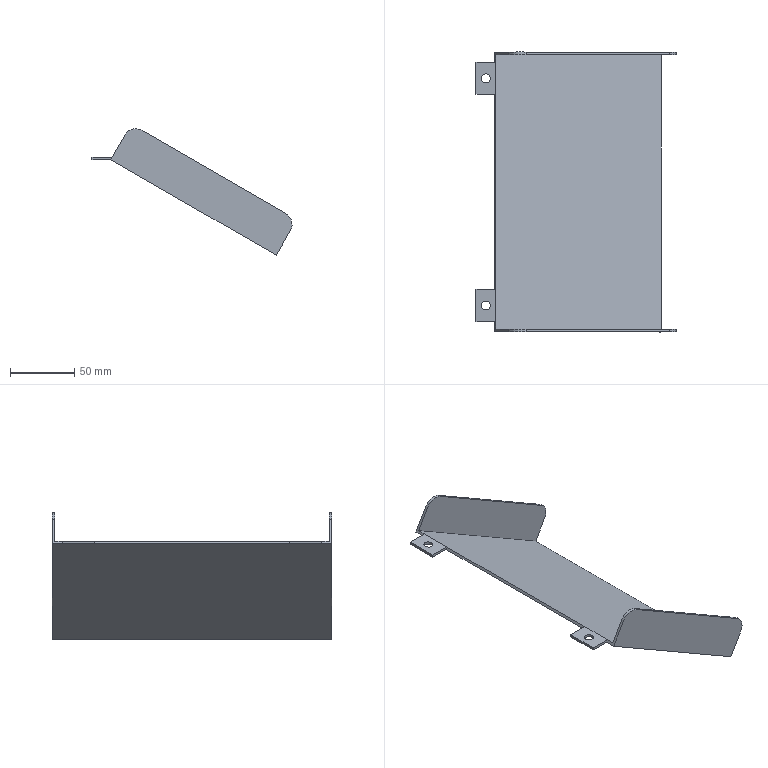Part | NX | features solid 2 | 1 solid | 30 faces | box 155.867 x 218 x 98.525 mm | volume 83984 mm3 | plane 24 | cylinder 6 | commonest cylinder face diameters 20 x4 7 x2
STEP:
#1=CARTESIAN_POINT('',(829.555,109.,-46.232));
#2=VERTEX_POINT('',#1);
#3=CARTESIAN_POINT('',(829.555,101.,-46.232));
#4=VERTEX_POINT('',#3);
#5=CARTESIAN_POINT('',(829.555,135.,-46.232));
#6=DIRECTION('',(0.,-1.,0.));
#7=VECTOR('',#6,1000.);
#8=LINE('',#5,#7);
#9=EDGE_CURVE('',#2,#4,#8,.T.);
#10=ORIENTED_EDGE('',*,*,#9,.T.);
#11=CARTESIAN_POINT('',(830.555,101.,-44.5));
#12=VERTEX_POINT('',#11);
#13=CARTESIAN_POINT('',(829.555,101.,-46.232));
#14=DIRECTION('',(-0.5,0.,-0.866));
#15=VECTOR('',#14,1000.);
#16=LINE('',#13,#15);
#17=EDGE_CURVE('',#4,#12,#16,.F.);
#18=ORIENTED_EDGE('',*,*,#17,.T.);
#19=CARTESIAN_POINT('',(830.555,107.,-44.5));
#20=VERTEX_POINT('',#19);
#21=CARTESIAN_POINT('',(830.555,135.,-44.5));
#22=DIRECTION('',(0.,-1.,0.));
#23=VECTOR('',#22,1000.);
#24=LINE('',#21,#23);
#25=EDGE_CURVE('',#20,#12,#24,.T.);
#26=ORIENTED_EDGE('',*,*,#25,.F.);
#27=CARTESIAN_POINT('',(840.555,107.,-27.179));
#28=VERTEX_POINT('',#27);
#29=CARTESIAN_POINT('',(830.555,107.,-44.5));
#30=DIRECTION('',(-0.5,0.,-0.866));
#31=VECTOR('',#30,1000.);
#32=LINE('',#29,#31);
#33=EDGE_CURVE('',#28,#20,#32,.T.);
#34=ORIENTED_EDGE('',*,*,#33,.F.);
#35=CARTESIAN_POINT('',(840.555,109.,-27.179));
#36=VERTEX_POINT('',#35);
#37=CARTESIAN_POINT('',(840.555,109.,-27.179));
#38=DIRECTION('',(0.,1.,0.));
#39=VECTOR('',#38,1000.);
#40=LINE('',#37,#39);
#41=EDGE_CURVE('',#28,#36,#40,.T.);
#42=ORIENTED_EDGE('',*,*,#41,.T.);
#43=CARTESIAN_POINT('',(830.555,109.,-44.5));
#44=DIRECTION('',(-0.5,0.,-0.866));
#45=VECTOR('',#44,1000.);
#46=LINE('',#43,#45);
#47=EDGE_CURVE('',#36,#2,#46,.T.);
#48=ORIENTED_EDGE('',*,*,#47,.T.);
#49=EDGE_LOOP('',(#10,#18,#26,#34,#42,#48));
#50=FACE_BOUND('',#49,.T.);
#51=CARTESIAN_POINT('',(829.555,99.,-46.232));
#52=DIRECTION('',(-0.866,0.,0.5));
#53=DIRECTION('',(0.5,0.,0.866));
#54=AXIS2_PLACEMENT_3D('',#51,#52,#53);
#55=PLANE('',#54);
#56=ADVANCED_FACE('',(#50),#55,.T.);
#57=CARTESIAN_POINT('',(829.555,76.,-46.232));
#58=VERTEX_POINT('',#57);
#59=CARTESIAN_POINT('',(830.555,76.,-44.5));
#60=VERTEX_POINT('',#59);
#61=CARTESIAN_POINT('',(827.39,76.,-49.982));
#62=DIRECTION('',(-0.5,0.,-0.866));
#63=VECTOR('',#62,1000.);
#64=LINE('',#61,#63);
#65=EDGE_CURVE('',#58,#60,#64,.F.);
#66=ORIENTED_EDGE('',*,*,#65,.F.);
#67=CARTESIAN_POINT('',(829.555,-76.,-46.232));
#68=VERTEX_POINT('',#67);
#69=CARTESIAN_POINT('',(829.555,135.,-46.232));
#70=DIRECTION('',(0.,-1.,0.));
#71=VECTOR('',#70,1000.);
#72=LINE('',#69,#71);
#73=EDGE_CURVE('',#58,#68,#72,.T.);
#74=ORIENTED_EDGE('',*,*,#73,.T.);
#75=CARTESIAN_POINT('',(830.555,-76.,-44.5));
#76=VERTEX_POINT('',#75);
#77=CARTESIAN_POINT('',(827.39,-76.,-49.982));
#78=DIRECTION('',(-0.5,0.,-0.866));
#79=VECTOR('',#78,1000.);
#80=LINE('',#77,#79);
#81=EDGE_CURVE('',#68,#76,#80,.F.);
#82=ORIENTED_EDGE('',*,*,#81,.T.);
#83=CARTESIAN_POINT('',(830.555,135.,-44.5));
#84=DIRECTION('',(0.,-1.,0.));
#85=VECTOR('',#84,1000.);
#86=LINE('',#83,#85);
#87=EDGE_CURVE('',#60,#76,#86,.T.);
#88=ORIENTED_EDGE('',*,*,#87,.F.);
#89=EDGE_LOOP('',(#66,#74,#82,#88));
#90=FACE_BOUND('',#89,.T.);
#91=CARTESIAN_POINT('',(829.555,99.,-46.232));
#92=DIRECTION('',(-0.866,0.,0.5));
#93=DIRECTION('',(0.5,0.,0.866));
#94=AXIS2_PLACEMENT_3D('',#91,#92,#93);
#95=PLANE('',#94);
#96=ADVANCED_FACE('',(#90),#95,.T.);
#97=ORIENTED_EDGE('',*,*,#47,.F.);
#98=CARTESIAN_POINT('',(854.215,109.,-23.519));
#99=VERTEX_POINT('',#98);
#100=CARTESIAN_POINT('',(849.215,109.,-32.179));
#101=DIRECTION('',(0.,-1.,0.));
#102=DIRECTION('',(0.,0.,-1.));
#103=AXIS2_PLACEMENT_3D('',#100,#101,#102);
#104=CIRCLE('',#103,10.);
#105=EDGE_CURVE('',#36,#99,#104,.F.);
#106=ORIENTED_EDGE('',*,*,#105,.T.);
#107=CARTESIAN_POINT('',(965.886,109.,-87.992));
#108=VERTEX_POINT('',#107);
#109=CARTESIAN_POINT('',(713.006,109.,58.008));
#110=DIRECTION('',(0.866,0.,-0.5));
#111=VECTOR('',#110,1000.);
#112=LINE('',#109,#111);
#113=EDGE_CURVE('',#99,#108,#112,.T.);
#114=ORIENTED_EDGE('',*,*,#113,.T.);
#115=CARTESIAN_POINT('',(969.546,109.,-101.652));
#116=VERTEX_POINT('',#115);
#117=CARTESIAN_POINT('',(960.886,109.,-96.652));
#118=DIRECTION('',(0.,-1.,0.));
#119=DIRECTION('',(0.08716,0.,0.9962));
#120=AXIS2_PLACEMENT_3D('',#117,#118,#119);
#121=CIRCLE('',#120,10.);
#122=EDGE_CURVE('',#108,#116,#121,.F.);
#123=ORIENTED_EDGE('',*,*,#122,.T.);
#124=CARTESIAN_POINT('',(958.546,109.,-120.705));
#125=VERTEX_POINT('',#124);
#126=CARTESIAN_POINT('',(959.546,109.,-118.973));
#127=DIRECTION('',(-0.5,0.,-0.866));
#128=VECTOR('',#127,1000.);
#129=LINE('',#126,#128);
#130=EDGE_CURVE('',#116,#125,#129,.T.);
#131=ORIENTED_EDGE('',*,*,#130,.T.);
#132=CARTESIAN_POINT('',(697.006,109.,30.295));
#133=DIRECTION('',(-0.866,0.,0.5));
#134=VECTOR('',#133,1000.);
#135=LINE('',#132,#134);
#136=EDGE_CURVE('',#125,#2,#135,.T.);
#137=ORIENTED_EDGE('',*,*,#136,.T.);
#138=EDGE_LOOP('',(#97,#106,#114,#123,#131,#137));
#139=FACE_BOUND('',#138,.T.);
#140=CARTESIAN_POINT('',(698.006,109.,32.027));
#141=DIRECTION('',(0.,-1.,0.));
#142=DIRECTION('',(0.08716,0.,0.9962));
#143=AXIS2_PLACEMENT_3D('',#140,#141,#142);
#144=PLANE('',#143);
#145=ADVANCED_FACE('',(#139),#144,.F.);
#146=CARTESIAN_POINT('',(854.215,-109.,-23.519));
#147=VERTEX_POINT('',#146);
#148=CARTESIAN_POINT('',(965.886,-109.,-87.992));
#149=VERTEX_POINT('',#148);
#150=CARTESIAN_POINT('',(713.006,-109.,58.008));
#151=DIRECTION('',(0.866,0.,-0.5));
#152=VECTOR('',#151,1000.);
#153=LINE('',#150,#152);
#154=EDGE_CURVE('',#147,#149,#153,.T.);
#155=ORIENTED_EDGE('',*,*,#154,.F.);
#156=CARTESIAN_POINT('',(840.555,-109.,-27.179));
#157=VERTEX_POINT('',#156);
#158=CARTESIAN_POINT('',(849.215,-109.,-32.179));
#159=DIRECTION('',(0.,1.,0.));
#160=DIRECTION('',(0.,0.,1.));
#161=AXIS2_PLACEMENT_3D('',#158,#159,#160);
#162=CIRCLE('',#161,10.);
#163=EDGE_CURVE('',#147,#157,#162,.F.);
#164=ORIENTED_EDGE('',*,*,#163,.T.);
#165=CARTESIAN_POINT('',(829.555,-109.,-46.232));
#166=VERTEX_POINT('',#165);
#167=CARTESIAN_POINT('',(830.555,-109.,-44.5));
#168=DIRECTION('',(0.5,0.,0.866));
#169=VECTOR('',#168,1000.);
#170=LINE('',#167,#169);
#171=EDGE_CURVE('',#166,#157,#170,.T.);
#172=ORIENTED_EDGE('',*,*,#171,.F.);
#173=CARTESIAN_POINT('',(958.546,-109.,-120.705));
#174=VERTEX_POINT('',#173);
#175=CARTESIAN_POINT('',(697.006,-109.,30.295));
#176=DIRECTION('',(0.866,0.,-0.5));
#177=VECTOR('',#176,1000.);
#178=LINE('',#175,#177);
#179=EDGE_CURVE('',#166,#174,#178,.T.);
#180=ORIENTED_EDGE('',*,*,#179,.T.);
#181=CARTESIAN_POINT('',(969.546,-109.,-101.652));
#182=VERTEX_POINT('',#181);
#183=CARTESIAN_POINT('',(959.546,-109.,-118.973));
#184=DIRECTION('',(-0.5,0.,-0.866));
#185=VECTOR('',#184,1000.);
#186=LINE('',#183,#185);
#187=EDGE_CURVE('',#182,#174,#186,.T.);
#188=ORIENTED_EDGE('',*,*,#187,.F.);
#189=CARTESIAN_POINT('',(960.886,-109.,-96.652));
#190=DIRECTION('',(0.,1.,0.));
#191=DIRECTION('',(-0.08716,0.,-0.9962));
#192=AXIS2_PLACEMENT_3D('',#189,#190,#191);
#193=CIRCLE('',#192,10.);
#194=EDGE_CURVE('',#182,#149,#193,.F.);
#195=ORIENTED_EDGE('',*,*,#194,.T.);
#196=EDGE_LOOP('',(#155,#164,#172,#180,#188,#195));
#197=FACE_BOUND('',#196,.T.);
#198=CARTESIAN_POINT('',(698.006,-109.,32.027));
#199=DIRECTION('',(0.,1.,0.));
#200=DIRECTION('',(-0.08716,0.,-0.9962));
#201=AXIS2_PLACEMENT_3D('',#198,#199,#200);
#202=PLANE('',#201);
#203=ADVANCED_FACE('',(#197),#202,.F.);
#204=CARTESIAN_POINT('',(830.555,-107.,-44.5));
#205=VERTEX_POINT('',#204);
#206=CARTESIAN_POINT('',(840.555,-107.,-27.179));
#207=VERTEX_POINT('',#206);
#208=CARTESIAN_POINT('',(830.555,-107.,-44.5));
#209=DIRECTION('',(0.5,0.,0.866));
#210=VECTOR('',#209,1000.);
#211=LINE('',#208,#210);
#212=EDGE_CURVE('',#205,#207,#211,.T.);
#213=ORIENTED_EDGE('',*,*,#212,.T.);
#214=CARTESIAN_POINT('',(854.215,-107.,-23.519));
#215=VERTEX_POINT('',#214);
#216=CARTESIAN_POINT('',(849.215,-107.,-32.179));
#217=DIRECTION('',(0.,1.,0.));
#218=DIRECTION('',(0.,0.,1.));
#219=AXIS2_PLACEMENT_3D('',#216,#217,#218);
#220=CIRCLE('',#219,10.);
#221=EDGE_CURVE('',#207,#215,#220,.T.);
#222=ORIENTED_EDGE('',*,*,#221,.T.);
#223=CARTESIAN_POINT('',(965.886,-107.,-87.992));
#224=VERTEX_POINT('',#223);
#225=CARTESIAN_POINT('',(713.006,-107.,58.008));
#226=DIRECTION('',(0.866,0.,-0.5));
#227=VECTOR('',#226,1000.);
#228=LINE('',#225,#227);
#229=EDGE_CURVE('',#215,#224,#228,.T.);
#230=ORIENTED_EDGE('',*,*,#229,.T.);
#231=CARTESIAN_POINT('',(969.546,-107.,-101.652));
#232=VERTEX_POINT('',#231);
#233=CARTESIAN_POINT('',(960.886,-107.,-96.652));
#234=DIRECTION('',(0.,1.,0.));
#235=DIRECTION('',(-0.08716,0.,-0.9962));
#236=AXIS2_PLACEMENT_3D('',#233,#234,#235);
#237=CIRCLE('',#236,10.);
#238=EDGE_CURVE('',#224,#232,#237,.T.);
#239=ORIENTED_EDGE('',*,*,#238,.T.);
#240=CARTESIAN_POINT('',(959.546,-107.,-118.973));
#241=VERTEX_POINT('',#240);
#242=CARTESIAN_POINT('',(959.546,-107.,-118.973));
#243=DIRECTION('',(-0.5,0.,-0.866));
#244=VECTOR('',#243,1000.);
#245=LINE('',#242,#244);
#246=EDGE_CURVE('',#232,#241,#245,.T.);
#247=ORIENTED_EDGE('',*,*,#246,.T.);
#248=CARTESIAN_POINT('',(698.006,-107.,32.027));
#249=DIRECTION('',(-0.866,0.,0.5));
#250=VECTOR('',#249,1000.);
#251=LINE('',#248,#250);
#252=EDGE_CURVE('',#241,#205,#251,.T.);
#253=ORIENTED_EDGE('',*,*,#252,.T.);
#254=EDGE_LOOP('',(#213,#222,#230,#239,#247,#253));
#255=FACE_BOUND('',#254,.T.);
#256=CARTESIAN_POINT('',(698.006,-107.,32.027));
#257=DIRECTION('',(0.,1.,0.));
#258=DIRECTION('',(-0.08716,0.,-0.9962));
#259=AXIS2_PLACEMENT_3D('',#256,#257,#258);
#260=PLANE('',#259);
#261=ADVANCED_FACE('',(#255),#260,.T.);
#262=CARTESIAN_POINT('',(854.215,107.,-23.519));
#263=VERTEX_POINT('',#262);
#264=CARTESIAN_POINT('',(965.886,107.,-87.992));
#265=VERTEX_POINT('',#264);
#266=CARTESIAN_POINT('',(713.006,107.,58.008));
#267=DIRECTION('',(0.866,0.,-0.5));
#268=VECTOR('',#267,1000.);
#269=LINE('',#266,#268);
#270=EDGE_CURVE('',#263,#265,#269,.T.);
#271=ORIENTED_EDGE('',*,*,#270,.F.);
#272=CARTESIAN_POINT('',(849.215,107.,-32.179));
#273=DIRECTION('',(0.,-1.,0.));
#274=DIRECTION('',(0.,0.,-1.));
#275=AXIS2_PLACEMENT_3D('',#272,#273,#274);
#276=CIRCLE('',#275,10.);
#277=EDGE_CURVE('',#263,#28,#276,.T.);
#278=ORIENTED_EDGE('',*,*,#277,.T.);
#279=ORIENTED_EDGE('',*,*,#33,.T.);
#280=CARTESIAN_POINT('',(959.546,107.,-118.973));
#281=VERTEX_POINT('',#280);
#282=CARTESIAN_POINT('',(698.006,107.,32.027));
#283=DIRECTION('',(0.866,0.,-0.5));
#284=VECTOR('',#283,1000.);
#285=LINE('',#282,#284);
#286=EDGE_CURVE('',#20,#281,#285,.T.);
#287=ORIENTED_EDGE('',*,*,#286,.T.);
#288=CARTESIAN_POINT('',(969.546,107.,-101.652));
#289=VERTEX_POINT('',#288);
#290=CARTESIAN_POINT('',(959.546,107.,-118.973));
#291=DIRECTION('',(-0.5,0.,-0.866));
#292=VECTOR('',#291,1000.);
#293=LINE('',#290,#292);
#294=EDGE_CURVE('',#289,#281,#293,.T.);
#295=ORIENTED_EDGE('',*,*,#294,.F.);
#296=CARTESIAN_POINT('',(960.886,107.,-96.652));
#297=DIRECTION('',(0.,-1.,0.));
#298=DIRECTION('',(0.08716,0.,0.9962));
#299=AXIS2_PLACEMENT_3D('',#296,#297,#298);
#300=CIRCLE('',#299,10.);
#301=EDGE_CURVE('',#289,#265,#300,.T.);
#302=ORIENTED_EDGE('',*,*,#301,.T.);
#303=EDGE_LOOP('',(#271,#278,#279,#287,#295,#302));
#304=FACE_BOUND('',#303,.T.);
#305=CARTESIAN_POINT('',(698.006,107.,32.027));
#306=DIRECTION('',(0.,-1.,0.));
#307=DIRECTION('',(-0.08716,0.,-0.9962));
#308=AXIS2_PLACEMENT_3D('',#305,#306,#307);
#309=PLANE('',#308);
#310=ADVANCED_FACE('',(#304),#309,.T.);
#311=ORIENTED_EDGE('',*,*,#229,.F.);
#312=CARTESIAN_POINT('',(854.215,-109.,-23.519));
#313=DIRECTION('',(0.,1.,0.));
#314=VECTOR('',#313,1000.);
#315=LINE('',#312,#314);
#316=EDGE_CURVE('',#215,#147,#315,.F.);
#317=ORIENTED_EDGE('',*,*,#316,.T.);
#318=ORIENTED_EDGE('',*,*,#154,.T.);
#319=CARTESIAN_POINT('',(965.886,-107.,-87.992));
#320=DIRECTION('',(0.,-1.,0.));
#321=VECTOR('',#320,1000.);
#322=LINE('',#319,#321);
#323=EDGE_CURVE('',#149,#224,#322,.F.);
#324=ORIENTED_EDGE('',*,*,#323,.T.);
#325=EDGE_LOOP('',(#311,#317,#318,#324));
#326=FACE_BOUND('',#325,.T.);
#327=CARTESIAN_POINT('',(713.006,-107.,58.008));
#328=DIRECTION('',(-0.5,0.,-0.866));
#329=DIRECTION('',(-0.866,0.,0.5));
#330=AXIS2_PLACEMENT_3D('',#327,#328,#329);
#331=PLANE('',#330);
#332=ADVANCED_FACE('',(#326),#331,.F.);
#333=ORIENTED_EDGE('',*,*,#113,.F.);
#334=CARTESIAN_POINT('',(854.215,107.,-23.519));
#335=DIRECTION('',(0.,1.,0.));
#336=VECTOR('',#335,1000.);
#337=LINE('',#334,#336);
#338=EDGE_CURVE('',#99,#263,#337,.F.);
#339=ORIENTED_EDGE('',*,*,#338,.T.);
#340=ORIENTED_EDGE('',*,*,#270,.T.);
#341=CARTESIAN_POINT('',(965.886,107.,-87.992));
#342=DIRECTION('',(0.,1.,0.));
#343=VECTOR('',#342,1000.);
#344=LINE('',#341,#343);
#345=EDGE_CURVE('',#265,#108,#344,.T.);
#346=ORIENTED_EDGE('',*,*,#345,.T.);
#347=EDGE_LOOP('',(#333,#339,#340,#346));
#348=FACE_BOUND('',#347,.T.);
#349=CARTESIAN_POINT('',(713.006,107.,58.008));
#350=DIRECTION('',(-0.5,0.,-0.866));
#351=DIRECTION('',(-0.866,0.,0.5));
#352=AXIS2_PLACEMENT_3D('',#349,#350,#351);
#353=PLANE('',#352);
#354=ADVANCED_FACE('',(#348),#353,.F.);
#355=ORIENTED_EDGE('',*,*,#286,.F.);
#356=ORIENTED_EDGE('',*,*,#25,.T.);
#357=CARTESIAN_POINT('',(830.555,99.,-44.5));
#358=DIRECTION('',(0.,1.,0.));
#359=VECTOR('',#358,1000.);
#360=LINE('',#357,#359);
#361=EDGE_CURVE('',#12,#60,#360,.F.);
#362=ORIENTED_EDGE('',*,*,#361,.T.);
#363=ORIENTED_EDGE('',*,*,#87,.T.);
#364=CARTESIAN_POINT('',(830.555,-101.,-44.5));
#365=VERTEX_POINT('',#364);
#366=CARTESIAN_POINT('',(830.555,-99.,-44.5));
#367=DIRECTION('',(0.,-1.,0.));
#368=VECTOR('',#367,1000.);
#369=LINE('',#366,#368);
#370=EDGE_CURVE('',#365,#76,#369,.F.);
#371=ORIENTED_EDGE('',*,*,#370,.F.);
#372=CARTESIAN_POINT('',(830.555,135.,-44.5));
#373=DIRECTION('',(0.,-1.,0.));
#374=VECTOR('',#373,1000.);
#375=LINE('',#372,#374);
#376=EDGE_CURVE('',#365,#205,#375,.T.);
#377=ORIENTED_EDGE('',*,*,#376,.T.);
#378=ORIENTED_EDGE('',*,*,#252,.F.);
#379=CARTESIAN_POINT('',(959.546,135.,-118.973));
#380=DIRECTION('',(0.,-1.,0.));
#381=VECTOR('',#380,1000.);
#382=LINE('',#379,#381);
#383=EDGE_CURVE('',#241,#281,#382,.F.);
#384=ORIENTED_EDGE('',*,*,#383,.T.);
#385=EDGE_LOOP('',(#355,#356,#362,#363,#371,#377,#378,#384));
#386=FACE_BOUND('',#385,.T.);
#387=CARTESIAN_POINT('',(698.006,135.,32.027));
#388=DIRECTION('',(0.5,0.,0.866));
#389=DIRECTION('',(0.,1.,0.));
#390=AXIS2_PLACEMENT_3D('',#387,#388,#389);
#391=PLANE('',#390);
#392=ADVANCED_FACE('',(#386),#391,.T.);
#393=ORIENTED_EDGE('',*,*,#9,.F.);
#394=ORIENTED_EDGE('',*,*,#136,.F.);
#395=CARTESIAN_POINT('',(958.546,135.,-120.705));
#396=DIRECTION('',(0.,-1.,0.));
#397=VECTOR('',#396,1000.);
#398=LINE('',#395,#397);
#399=EDGE_CURVE('',#174,#125,#398,.F.);
#400=ORIENTED_EDGE('',*,*,#399,.F.);
#401=ORIENTED_EDGE('',*,*,#179,.F.);
#402=CARTESIAN_POINT('',(829.555,-101.,-46.232));
#403=VERTEX_POINT('',#402);
#404=CARTESIAN_POINT('',(829.555,135.,-46.232));
#405=DIRECTION('',(0.,-1.,0.));
#406=VECTOR('',#405,1000.);
#407=LINE('',#404,#406);
#408=EDGE_CURVE('',#403,#166,#407,.T.);
#409=ORIENTED_EDGE('',*,*,#408,.F.);
#410=CARTESIAN_POINT('',(829.555,135.,-46.232));
#411=DIRECTION('',(0.,-1.,0.));
#412=VECTOR('',#411,1000.);
#413=LINE('',#410,#412);
#414=EDGE_CURVE('',#68,#403,#413,.T.);
#415=ORIENTED_EDGE('',*,*,#414,.F.);
#416=ORIENTED_EDGE('',*,*,#73,.F.);
#417=CARTESIAN_POINT('',(829.555,135.,-46.232));
#418=DIRECTION('',(0.,-1.,0.));
#419=VECTOR('',#418,1000.);
#420=LINE('',#417,#419);
#421=EDGE_CURVE('',#4,#58,#420,.T.);
#422=ORIENTED_EDGE('',*,*,#421,.F.);
#423=EDGE_LOOP('',(#393,#394,#400,#401,#409,#415,#416,#422));
#424=FACE_BOUND('',#423,.T.);
#425=CARTESIAN_POINT('',(697.006,135.,30.295));
#426=DIRECTION('',(0.5,0.,0.866));
#427=DIRECTION('',(0.,1.,0.));
#428=AXIS2_PLACEMENT_3D('',#425,#426,#427);
#429=PLANE('',#428);
#430=ADVANCED_FACE('',(#424),#429,.F.);
#431=ORIENTED_EDGE('',*,*,#130,.F.);
#432=CARTESIAN_POINT('',(969.546,135.,-101.652));
#433=DIRECTION('',(0.,1.,0.));
#434=VECTOR('',#433,1000.);
#435=LINE('',#432,#434);
#436=EDGE_CURVE('',#116,#289,#435,.F.);
#437=ORIENTED_EDGE('',*,*,#436,.T.);
#438=ORIENTED_EDGE('',*,*,#294,.T.);
#439=ORIENTED_EDGE('',*,*,#383,.F.);
#440=ORIENTED_EDGE('',*,*,#246,.F.);
#441=CARTESIAN_POINT('',(969.546,135.,-101.652));
#442=DIRECTION('',(0.,-1.,0.));
#443=VECTOR('',#442,1000.);
#444=LINE('',#441,#443);
#445=EDGE_CURVE('',#232,#182,#444,.T.);
#446=ORIENTED_EDGE('',*,*,#445,.T.);
#447=ORIENTED_EDGE('',*,*,#187,.T.);
#448=ORIENTED_EDGE('',*,*,#399,.T.);
#449=EDGE_LOOP('',(#431,#437,#438,#439,#440,#446,#447,#448));
#450=FACE_BOUND('',#449,.T.);
#451=CARTESIAN_POINT('',(959.546,135.,-118.973));
#452=DIRECTION('',(-0.866,0.,0.5));
#453=DIRECTION('',(0.5,0.,0.866));
#454=AXIS2_PLACEMENT_3D('',#451,#452,#453);
#455=PLANE('',#454);
#456=ADVANCED_FACE('',(#450),#455,.F.);
#457=ORIENTED_EDGE('',*,*,#301,.F.);
#458=ORIENTED_EDGE('',*,*,#436,.F.);
#459=ORIENTED_EDGE('',*,*,#122,.F.);
#460=ORIENTED_EDGE('',*,*,#345,.F.);
#461=EDGE_LOOP('',(#457,#458,#459,#460));
#462=FACE_BOUND('',#461,.T.);
#463=CARTESIAN_POINT('',(960.886,107.,-96.652));
#464=DIRECTION('',(0.,1.,0.));
#465=DIRECTION('',(-0.08716,0.,-0.9962));
#466=AXIS2_PLACEMENT_3D('',#463,#464,#465);
#467=CYLINDRICAL_SURFACE('',#466,10.);
#468=ADVANCED_FACE('',(#462),#467,.T.);
#469=ORIENTED_EDGE('',*,*,#238,.F.);
#470=ORIENTED_EDGE('',*,*,#323,.F.);
#471=ORIENTED_EDGE('',*,*,#194,.F.);
#472=ORIENTED_EDGE('',*,*,#445,.F.);
#473=EDGE_LOOP('',(#469,#470,#471,#472));
#474=FACE_BOUND('',#473,.T.);
#475=CARTESIAN_POINT('',(960.886,151.,-96.652));
#476=DIRECTION('',(0.,-1.,0.));
#477=DIRECTION('',(0.08716,0.,0.9962));
#478=AXIS2_PLACEMENT_3D('',#475,#476,#477);
#479=CYLINDRICAL_SURFACE('',#478,10.);
#480=ADVANCED_FACE('',(#474),#479,.T.);
#481=CARTESIAN_POINT('',(829.555,-101.,-46.232));
#482=DIRECTION('',(-0.5,0.,-0.866));
#483=VECTOR('',#482,1000.);
#484=LINE('',#481,#483);
#485=EDGE_CURVE('',#403,#365,#484,.F.);
#486=ORIENTED_EDGE('',*,*,#485,.F.);
#487=ORIENTED_EDGE('',*,*,#408,.T.);
#488=ORIENTED_EDGE('',*,*,#171,.T.);
#489=CARTESIAN_POINT('',(840.555,-107.,-27.179));
#490=DIRECTION('',(0.,1.,0.));
#491=VECTOR('',#490,1000.);
#492=LINE('',#489,#491);
#493=EDGE_CURVE('',#157,#207,#492,.T.);
#494=ORIENTED_EDGE('',*,*,#493,.T.);
#495=ORIENTED_EDGE('',*,*,#212,.F.);
#496=ORIENTED_EDGE('',*,*,#376,.F.);
#497=EDGE_LOOP('',(#486,#487,#488,#494,#495,#496));
#498=FACE_BOUND('',#497,.T.);
#499=CARTESIAN_POINT('',(829.555,99.,-46.232));
#500=DIRECTION('',(-0.866,0.,0.5));
#501=DIRECTION('',(0.5,0.,0.866));
#502=AXIS2_PLACEMENT_3D('',#499,#500,#501);
#503=PLANE('',#502);
#504=ADVANCED_FACE('',(#498),#503,.T.);
#505=ORIENTED_EDGE('',*,*,#277,.F.);
#506=ORIENTED_EDGE('',*,*,#338,.F.);
#507=ORIENTED_EDGE('',*,*,#105,.F.);
#508=ORIENTED_EDGE('',*,*,#41,.F.);
#509=EDGE_LOOP('',(#505,#506,#507,#508));
#510=FACE_BOUND('',#509,.T.);
#511=CARTESIAN_POINT('',(849.215,109.,-32.179));
#512=DIRECTION('',(0.,-1.,0.));
#513=DIRECTION('',(0.,0.,-1.));
#514=AXIS2_PLACEMENT_3D('',#511,#512,#513);
#515=CYLINDRICAL_SURFACE('',#514,10.);
#516=ADVANCED_FACE('',(#510),#515,.T.);
#517=ORIENTED_EDGE('',*,*,#163,.F.);
#518=ORIENTED_EDGE('',*,*,#316,.F.);
#519=ORIENTED_EDGE('',*,*,#221,.F.);
#520=ORIENTED_EDGE('',*,*,#493,.F.);
#521=EDGE_LOOP('',(#517,#518,#519,#520));
#522=FACE_BOUND('',#521,.T.);
#523=CARTESIAN_POINT('',(849.215,89.,-32.179));
#524=DIRECTION('',(0.,-1.,0.));
#525=DIRECTION('',(0.,0.,-1.));
#526=AXIS2_PLACEMENT_3D('',#523,#524,#525);
#527=CYLINDRICAL_SURFACE('',#526,10.);
#528=ADVANCED_FACE('',(#522),#527,.T.);
#529=CARTESIAN_POINT('',(819.287,-88.5,-46.5));
#530=VERTEX_POINT('',#529);
#531=CARTESIAN_POINT('',(822.787,-88.5,-46.5));
#532=DIRECTION('',(0.,0.,1.));
#533=DIRECTION('',(-1.,0.,0.));
#534=AXIS2_PLACEMENT_3D('',#531,#532,#533);
#535=CIRCLE('',#534,3.5);
#536=EDGE_CURVE('',#530,#530,#535,.T.);
#537=ORIENTED_EDGE('',*,*,#536,.T.);
#538=EDGE_LOOP('',(#537));
#539=FACE_BOUND('',#538,.T.);
#540=CARTESIAN_POINT('',(815.019,-76.,-46.5));
#541=VERTEX_POINT('',#540);
#542=CARTESIAN_POINT('',(829.4,-76.,-46.5));
#543=VERTEX_POINT('',#542);
#544=CARTESIAN_POINT('',(830.019,-76.,-46.5));
#545=DIRECTION('',(1.,0.,0.));
#546=VECTOR('',#545,1000.);
#547=LINE('',#544,#546);
#548=EDGE_CURVE('',#541,#543,#547,.T.);
#549=ORIENTED_EDGE('',*,*,#548,.T.);
#550=CARTESIAN_POINT('',(829.4,-101.,-46.5));
#551=VERTEX_POINT('',#550);
#552=CARTESIAN_POINT('',(829.4,-99.,-46.5));
#553=DIRECTION('',(0.,1.,0.));
#554=VECTOR('',#553,1000.);
#555=LINE('',#552,#554);
#556=EDGE_CURVE('',#543,#551,#555,.F.);
#557=ORIENTED_EDGE('',*,*,#556,.T.);
#558=CARTESIAN_POINT('',(815.019,-101.,-46.5));
#559=VERTEX_POINT('',#558);
#560=CARTESIAN_POINT('',(830.019,-101.,-46.5));
#561=DIRECTION('',(-1.,0.,0.));
#562=VECTOR('',#561,1000.);
#563=LINE('',#560,#562);
#564=EDGE_CURVE('',#551,#559,#563,.T.);
#565=ORIENTED_EDGE('',*,*,#564,.T.);
#566=CARTESIAN_POINT('',(815.019,-96.,-46.5));
#567=DIRECTION('',(0.,1.,0.));
#568=VECTOR('',#567,1000.);
#569=LINE('',#566,#568);
#570=EDGE_CURVE('',#559,#541,#569,.T.);
#571=ORIENTED_EDGE('',*,*,#570,.T.);
#572=EDGE_LOOP('',(#549,#557,#565,#571));
#573=FACE_BOUND('',#572,.T.);
#574=CARTESIAN_POINT('',(276.,0.,-46.5));
#575=DIRECTION('',(0.,0.,-1.));
#576=DIRECTION('',(-1.,0.,0.));
#577=AXIS2_PLACEMENT_3D('',#574,#575,#576);
#578=PLANE('',#577);
#579=ADVANCED_FACE('',(#539,#573),#578,.T.);
#580=CARTESIAN_POINT('',(815.019,-76.,-44.5));
#581=VERTEX_POINT('',#580);
#582=CARTESIAN_POINT('',(815.019,-76.,-51.5));
#583=DIRECTION('',(0.,0.,1.));
#584=VECTOR('',#583,1000.);
#585=LINE('',#582,#584);
#586=EDGE_CURVE('',#541,#581,#585,.T.);
#587=ORIENTED_EDGE('',*,*,#586,.T.);
#588=CARTESIAN_POINT('',(830.019,-76.,-44.5));
#589=DIRECTION('',(-1.,0.,0.));
#590=VECTOR('',#589,1000.);
#591=LINE('',#588,#590);
#592=EDGE_CURVE('',#76,#581,#591,.T.);
#593=ORIENTED_EDGE('',*,*,#592,.F.);
#594=ORIENTED_EDGE('',*,*,#81,.F.);
#595=CARTESIAN_POINT('',(827.39,-76.,-49.982));
#596=DIRECTION('',(-0.5,0.,-0.866));
#597=VECTOR('',#596,1000.);
#598=LINE('',#595,#597);
#599=EDGE_CURVE('',#543,#68,#598,.F.);
#600=ORIENTED_EDGE('',*,*,#599,.F.);
#601=ORIENTED_EDGE('',*,*,#548,.F.);
#602=EDGE_LOOP('',(#587,#593,#594,#600,#601));
#603=FACE_BOUND('',#602,.T.);
#604=CARTESIAN_POINT('',(830.019,-76.,-51.5));
#605=DIRECTION('',(0.,1.,0.));
#606=DIRECTION('',(0.,0.,-1.));
#607=AXIS2_PLACEMENT_3D('',#604,#605,#606);
#608=PLANE('',#607);
#609=ADVANCED_FACE('',(#603),#608,.T.);
#610=CARTESIAN_POINT('',(815.019,-101.,-44.5));
#611=VERTEX_POINT('',#610);
#612=CARTESIAN_POINT('',(815.019,-101.,-51.5));
#613=DIRECTION('',(0.,0.,1.));
#614=VECTOR('',#613,1000.);
#615=LINE('',#612,#614);
#616=EDGE_CURVE('',#559,#611,#615,.T.);
#617=ORIENTED_EDGE('',*,*,#616,.T.);
#618=CARTESIAN_POINT('',(815.019,-96.,-44.5));
#619=DIRECTION('',(0.,-1.,0.));
#620=VECTOR('',#619,1000.);
#621=LINE('',#618,#620);
#622=EDGE_CURVE('',#581,#611,#621,.T.);
#623=ORIENTED_EDGE('',*,*,#622,.F.);
#624=ORIENTED_EDGE('',*,*,#586,.F.);
#625=ORIENTED_EDGE('',*,*,#570,.F.);
#626=EDGE_LOOP('',(#617,#623,#624,#625));
#627=FACE_BOUND('',#626,.T.);
#628=CARTESIAN_POINT('',(815.019,-96.,-51.5));
#629=DIRECTION('',(-1.,0.,0.));
#630=DIRECTION('',(0.,0.,1.));
#631=AXIS2_PLACEMENT_3D('',#628,#629,#630);
#632=PLANE('',#631);
#633=ADVANCED_FACE('',(#627),#632,.T.);
#634=CARTESIAN_POINT('',(829.555,-101.,-46.232));
#635=DIRECTION('',(-0.5,0.,-0.866));
#636=VECTOR('',#635,1000.);
#637=LINE('',#634,#636);
#638=EDGE_CURVE('',#551,#403,#637,.F.);
#639=ORIENTED_EDGE('',*,*,#638,.T.);
#640=ORIENTED_EDGE('',*,*,#485,.T.);
#641=CARTESIAN_POINT('',(830.019,-101.,-44.5));
#642=DIRECTION('',(1.,0.,0.));
#643=VECTOR('',#642,1000.);
#644=LINE('',#641,#643);
#645=EDGE_CURVE('',#611,#365,#644,.T.);
#646=ORIENTED_EDGE('',*,*,#645,.F.);
#647=ORIENTED_EDGE('',*,*,#616,.F.);
#648=ORIENTED_EDGE('',*,*,#564,.F.);
#649=EDGE_LOOP('',(#639,#640,#646,#647,#648));
#650=FACE_BOUND('',#649,.T.);
#651=CARTESIAN_POINT('',(830.019,-101.,-51.5));
#652=DIRECTION('',(0.,-1.,0.));
#653=DIRECTION('',(0.,0.,1.));
#654=AXIS2_PLACEMENT_3D('',#651,#652,#653);
#655=PLANE('',#654);
#656=ADVANCED_FACE('',(#650),#655,.T.);
#657=ORIENTED_EDGE('',*,*,#599,.T.);
#658=ORIENTED_EDGE('',*,*,#414,.T.);
#659=ORIENTED_EDGE('',*,*,#638,.F.);
#660=ORIENTED_EDGE('',*,*,#556,.F.);
#661=EDGE_LOOP('',(#657,#658,#659,#660));
#662=FACE_BOUND('',#661,.T.);
#663=CARTESIAN_POINT('',(829.555,-99.,-46.232));
#664=DIRECTION('',(-0.866,0.,0.5));
#665=DIRECTION('',(0.5,0.,0.866));
#666=AXIS2_PLACEMENT_3D('',#663,#664,#665);
#667=PLANE('',#666);
#668=ADVANCED_FACE('',(#662),#667,.F.);
#669=ORIENTED_EDGE('',*,*,#592,.T.);
#670=ORIENTED_EDGE('',*,*,#622,.T.);
#671=ORIENTED_EDGE('',*,*,#645,.T.);
#672=ORIENTED_EDGE('',*,*,#370,.T.);
#673=EDGE_LOOP('',(#669,#670,#671,#672));
#674=FACE_BOUND('',#673,.T.);
#675=CARTESIAN_POINT('',(819.287,-88.5,-44.5));
#676=VERTEX_POINT('',#675);
#677=CARTESIAN_POINT('',(822.787,-88.5,-44.5));
#678=DIRECTION('',(0.,0.,1.));
#679=DIRECTION('',(-1.,0.,0.));
#680=AXIS2_PLACEMENT_3D('',#677,#678,#679);
#681=CIRCLE('',#680,3.5);
#682=EDGE_CURVE('',#676,#676,#681,.F.);
#683=ORIENTED_EDGE('',*,*,#682,.T.);
#684=EDGE_LOOP('',(#683));
#685=FACE_BOUND('',#684,.T.);
#686=CARTESIAN_POINT('',(830.019,-96.,-44.5));
#687=DIRECTION('',(0.,0.,1.));
#688=DIRECTION('',(1.,0.,0.));
#689=AXIS2_PLACEMENT_3D('',#686,#687,#688);
#690=PLANE('',#689);
#691=ADVANCED_FACE('',(#674,#685),#690,.T.);
#692=ORIENTED_EDGE('',*,*,#536,.F.);
#693=EDGE_LOOP('',(#692));
#694=FACE_BOUND('',#693,.T.);
#695=ORIENTED_EDGE('',*,*,#682,.F.);
#696=EDGE_LOOP('',(#695));
#697=FACE_BOUND('',#696,.T.);
#698=CARTESIAN_POINT('',(822.787,-88.5,-35.5));
#699=DIRECTION('',(0.,0.,-1.));
#700=DIRECTION('',(1.,0.,0.));
#701=AXIS2_PLACEMENT_3D('',#698,#699,#700);
#702=CYLINDRICAL_SURFACE('',#701,3.5);
#703=ADVANCED_FACE('',(#694,#697),#702,.F.);
#704=CARTESIAN_POINT('',(819.287,88.5,-46.5));
#705=VERTEX_POINT('',#704);
#706=CARTESIAN_POINT('',(822.787,88.5,-46.5));
#707=DIRECTION('',(0.,0.,-1.));
#708=DIRECTION('',(-1.,0.,0.));
#709=AXIS2_PLACEMENT_3D('',#706,#707,#708);
#710=CIRCLE('',#709,3.5);
#711=EDGE_CURVE('',#705,#705,#710,.T.);
#712=ORIENTED_EDGE('',*,*,#711,.F.);
#713=EDGE_LOOP('',(#712));
#714=FACE_BOUND('',#713,.T.);
#715=CARTESIAN_POINT('',(815.019,76.,-46.5));
#716=VERTEX_POINT('',#715);
#717=CARTESIAN_POINT('',(829.4,76.,-46.5));
#718=VERTEX_POINT('',#717);
#719=CARTESIAN_POINT('',(830.019,76.,-46.5));
#720=DIRECTION('',(1.,0.,0.));
#721=VECTOR('',#720,1000.);
#722=LINE('',#719,#721);
#723=EDGE_CURVE('',#716,#718,#722,.T.);
#724=ORIENTED_EDGE('',*,*,#723,.F.);
#725=CARTESIAN_POINT('',(815.019,101.,-46.5));
#726=VERTEX_POINT('',#725);
#727=CARTESIAN_POINT('',(815.019,96.,-46.5));
#728=DIRECTION('',(0.,-1.,0.));
#729=VECTOR('',#728,1000.);
#730=LINE('',#727,#729);
#731=EDGE_CURVE('',#726,#716,#730,.T.);
#732=ORIENTED_EDGE('',*,*,#731,.F.);
#733=CARTESIAN_POINT('',(829.4,101.,-46.5));
#734=VERTEX_POINT('',#733);
#735=CARTESIAN_POINT('',(830.019,101.,-46.5));
#736=DIRECTION('',(-1.,0.,0.));
#737=VECTOR('',#736,1000.);
#738=LINE('',#735,#737);
#739=EDGE_CURVE('',#734,#726,#738,.T.);
#740=ORIENTED_EDGE('',*,*,#739,.F.);
#741=CARTESIAN_POINT('',(829.4,99.,-46.5));
#742=DIRECTION('',(0.,-1.,0.));
#743=VECTOR('',#742,1000.);
#744=LINE('',#741,#743);
#745=EDGE_CURVE('',#718,#734,#744,.F.);
#746=ORIENTED_EDGE('',*,*,#745,.F.);
#747=EDGE_LOOP('',(#724,#732,#740,#746));
#748=FACE_BOUND('',#747,.T.);
#749=CARTESIAN_POINT('',(276.,0.,-46.5));
#750=DIRECTION('',(0.,0.,-1.));
#751=DIRECTION('',(-1.,0.,0.));
#752=AXIS2_PLACEMENT_3D('',#749,#750,#751);
#753=PLANE('',#752);
#754=ADVANCED_FACE('',(#714,#748),#753,.T.);
#755=CARTESIAN_POINT('',(815.019,76.,-44.5));
#756=VERTEX_POINT('',#755);
#757=CARTESIAN_POINT('',(815.019,76.,-51.5));
#758=DIRECTION('',(0.,0.,1.));
#759=VECTOR('',#758,1000.);
#760=LINE('',#757,#759);
#761=EDGE_CURVE('',#716,#756,#760,.T.);
#762=ORIENTED_EDGE('',*,*,#761,.F.);
#763=ORIENTED_EDGE('',*,*,#723,.T.);
#764=CARTESIAN_POINT('',(827.39,76.,-49.982));
#765=DIRECTION('',(-0.5,0.,-0.866));
#766=VECTOR('',#765,1000.);
#767=LINE('',#764,#766);
#768=EDGE_CURVE('',#718,#58,#767,.F.);
#769=ORIENTED_EDGE('',*,*,#768,.T.);
#770=ORIENTED_EDGE('',*,*,#65,.T.);
#771=CARTESIAN_POINT('',(830.019,76.,-44.5));
#772=DIRECTION('',(-1.,0.,0.));
#773=VECTOR('',#772,1000.);
#774=LINE('',#771,#773);
#775=EDGE_CURVE('',#60,#756,#774,.T.);
#776=ORIENTED_EDGE('',*,*,#775,.T.);
#777=EDGE_LOOP('',(#762,#763,#769,#770,#776));
#778=FACE_BOUND('',#777,.T.);
#779=CARTESIAN_POINT('',(830.019,76.,-51.5));
#780=DIRECTION('',(0.,-1.,0.));
#781=DIRECTION('',(0.,0.,-1.));
#782=AXIS2_PLACEMENT_3D('',#779,#780,#781);
#783=PLANE('',#782);
#784=ADVANCED_FACE('',(#778),#783,.T.);
#785=CARTESIAN_POINT('',(815.019,101.,-44.5));
#786=VERTEX_POINT('',#785);
#787=CARTESIAN_POINT('',(815.019,101.,-51.5));
#788=DIRECTION('',(0.,0.,1.));
#789=VECTOR('',#788,1000.);
#790=LINE('',#787,#789);
#791=EDGE_CURVE('',#726,#786,#790,.T.);
#792=ORIENTED_EDGE('',*,*,#791,.F.);
#793=ORIENTED_EDGE('',*,*,#731,.T.);
#794=ORIENTED_EDGE('',*,*,#761,.T.);
#795=CARTESIAN_POINT('',(815.019,96.,-44.5));
#796=DIRECTION('',(0.,1.,0.));
#797=VECTOR('',#796,1000.);
#798=LINE('',#795,#797);
#799=EDGE_CURVE('',#756,#786,#798,.T.);
#800=ORIENTED_EDGE('',*,*,#799,.T.);
#801=EDGE_LOOP('',(#792,#793,#794,#800));
#802=FACE_BOUND('',#801,.T.);
#803=CARTESIAN_POINT('',(815.019,96.,-51.5));
#804=DIRECTION('',(-1.,0.,0.));
#805=DIRECTION('',(0.,0.,1.));
#806=AXIS2_PLACEMENT_3D('',#803,#804,#805);
#807=PLANE('',#806);
#808=ADVANCED_FACE('',(#802),#807,.T.);
#809=CARTESIAN_POINT('',(829.555,101.,-46.232));
#810=DIRECTION('',(-0.5,0.,-0.866));
#811=VECTOR('',#810,1000.);
#812=LINE('',#809,#811);
#813=EDGE_CURVE('',#734,#4,#812,.F.);
#814=ORIENTED_EDGE('',*,*,#813,.F.);
#815=ORIENTED_EDGE('',*,*,#739,.T.);
#816=ORIENTED_EDGE('',*,*,#791,.T.);
#817=CARTESIAN_POINT('',(830.019,101.,-44.5));
#818=DIRECTION('',(1.,0.,0.));
#819=VECTOR('',#818,1000.);
#820=LINE('',#817,#819);
#821=EDGE_CURVE('',#786,#12,#820,.T.);
#822=ORIENTED_EDGE('',*,*,#821,.T.);
#823=ORIENTED_EDGE('',*,*,#17,.F.);
#824=EDGE_LOOP('',(#814,#815,#816,#822,#823));
#825=FACE_BOUND('',#824,.T.);
#826=CARTESIAN_POINT('',(830.019,101.,-51.5));
#827=DIRECTION('',(0.,1.,0.));
#828=DIRECTION('',(0.,0.,1.));
#829=AXIS2_PLACEMENT_3D('',#826,#827,#828);
#830=PLANE('',#829);
#831=ADVANCED_FACE('',(#825),#830,.T.);
#832=ORIENTED_EDGE('',*,*,#813,.T.);
#833=ORIENTED_EDGE('',*,*,#421,.T.);
#834=ORIENTED_EDGE('',*,*,#768,.F.);
#835=ORIENTED_EDGE('',*,*,#745,.T.);
#836=EDGE_LOOP('',(#832,#833,#834,#835));
#837=FACE_BOUND('',#836,.T.);
#838=CARTESIAN_POINT('',(829.555,99.,-46.232));
#839=DIRECTION('',(-0.866,0.,0.5));
#840=DIRECTION('',(0.5,0.,0.866));
#841=AXIS2_PLACEMENT_3D('',#838,#839,#840);
#842=PLANE('',#841);
#843=ADVANCED_FACE('',(#837),#842,.F.);
#844=ORIENTED_EDGE('',*,*,#775,.F.);
#845=ORIENTED_EDGE('',*,*,#361,.F.);
#846=ORIENTED_EDGE('',*,*,#821,.F.);
#847=ORIENTED_EDGE('',*,*,#799,.F.);
#848=EDGE_LOOP('',(#844,#845,#846,#847));
#849=FACE_BOUND('',#848,.T.);
#850=CARTESIAN_POINT('',(819.287,88.5,-44.5));
#851=VERTEX_POINT('',#850);
#852=CARTESIAN_POINT('',(822.787,88.5,-44.5));
#853=DIRECTION('',(0.,0.,-1.));
#854=DIRECTION('',(-1.,0.,0.));
#855=AXIS2_PLACEMENT_3D('',#852,#853,#854);
#856=CIRCLE('',#855,3.5);
#857=EDGE_CURVE('',#851,#851,#856,.F.);
#858=ORIENTED_EDGE('',*,*,#857,.F.);
#859=EDGE_LOOP('',(#858));
#860=FACE_BOUND('',#859,.T.);
#861=CARTESIAN_POINT('',(830.019,96.,-44.5));
#862=DIRECTION('',(0.,0.,1.));
#863=DIRECTION('',(1.,0.,0.));
#864=AXIS2_PLACEMENT_3D('',#861,#862,#863);
#865=PLANE('',#864);
#866=ADVANCED_FACE('',(#849,#860),#865,.T.);
#867=ORIENTED_EDGE('',*,*,#711,.T.);
#868=EDGE_LOOP('',(#867));
#869=FACE_BOUND('',#868,.T.);
#870=ORIENTED_EDGE('',*,*,#857,.T.);
#871=EDGE_LOOP('',(#870));
#872=FACE_BOUND('',#871,.T.);
#873=CARTESIAN_POINT('',(822.787,88.5,-35.5));
#874=DIRECTION('',(0.,0.,-1.));
#875=DIRECTION('',(1.,0.,0.));
#876=AXIS2_PLACEMENT_3D('',#873,#874,#875);
#877=CYLINDRICAL_SURFACE('',#876,3.5);
#878=ADVANCED_FACE('',(#869,#872),#877,.F.);
#879=CLOSED_SHELL('',(#56,#96,#145,#203,#261,#310,#332,#354,#392,#430,#456,#468,#480,#504,#516,#528,#579,#609,#633,#656,#668,#691,#703,#754,#784,#808,#831,#843,#866,#878));
#880=MANIFOLD_SOLID_BREP('',#879);
#881=(LENGTH_UNIT()NAMED_UNIT(*)SI_UNIT(.MILLI.,.METRE.));
#882=UNCERTAINTY_MEASURE_WITH_UNIT(LENGTH_MEASURE(0.00001),#881,'','');
#883=(NAMED_UNIT(*)PLANE_ANGLE_UNIT()SI_UNIT($,.RADIAN.));
#884=(NAMED_UNIT(*)SI_UNIT($,.STERADIAN.)SOLID_ANGLE_UNIT());
#885=(GEOMETRIC_REPRESENTATION_CONTEXT(3)GLOBAL_UNCERTAINTY_ASSIGNED_CONTEXT((#882))GLOBAL_UNIT_ASSIGNED_CONTEXT((#881,#883,#884))REPRESENTATION_CONTEXT('',''));
#886=ADVANCED_BREP_SHAPE_REPRESENTATION('',(#880),#885);